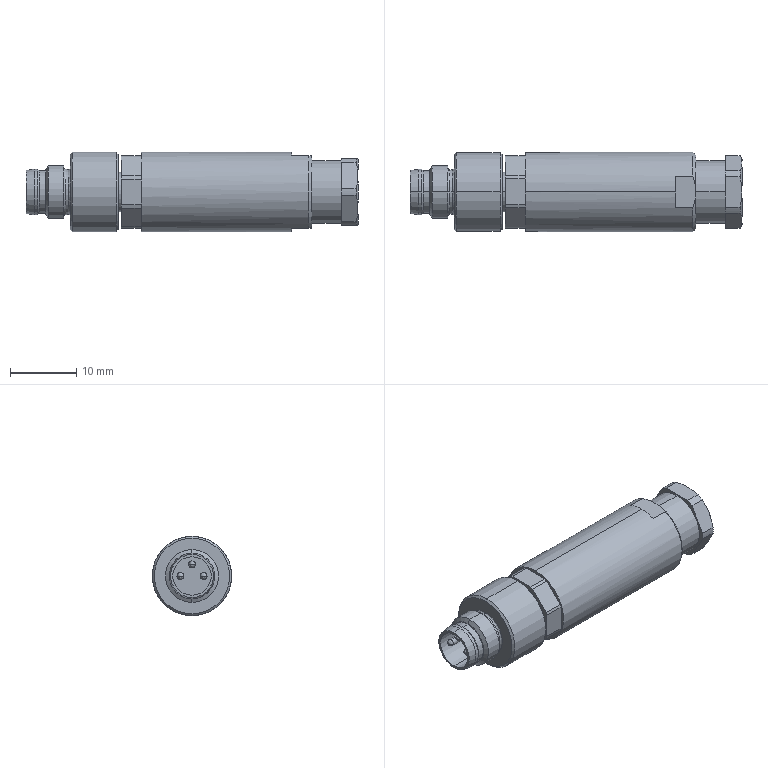Part | SolidWorks | features BaseBody 1 | 1 solid | 95 faces | box 50.1 x 12 x 12 mm | volume 4699 mm3 | plane 37 | cylinder 30 | cone 18 | spline 10 | commonest cylinder face diameters 1.03 x6 11 x6 12 x4 5.8 x2 6 x2 6.5 x2